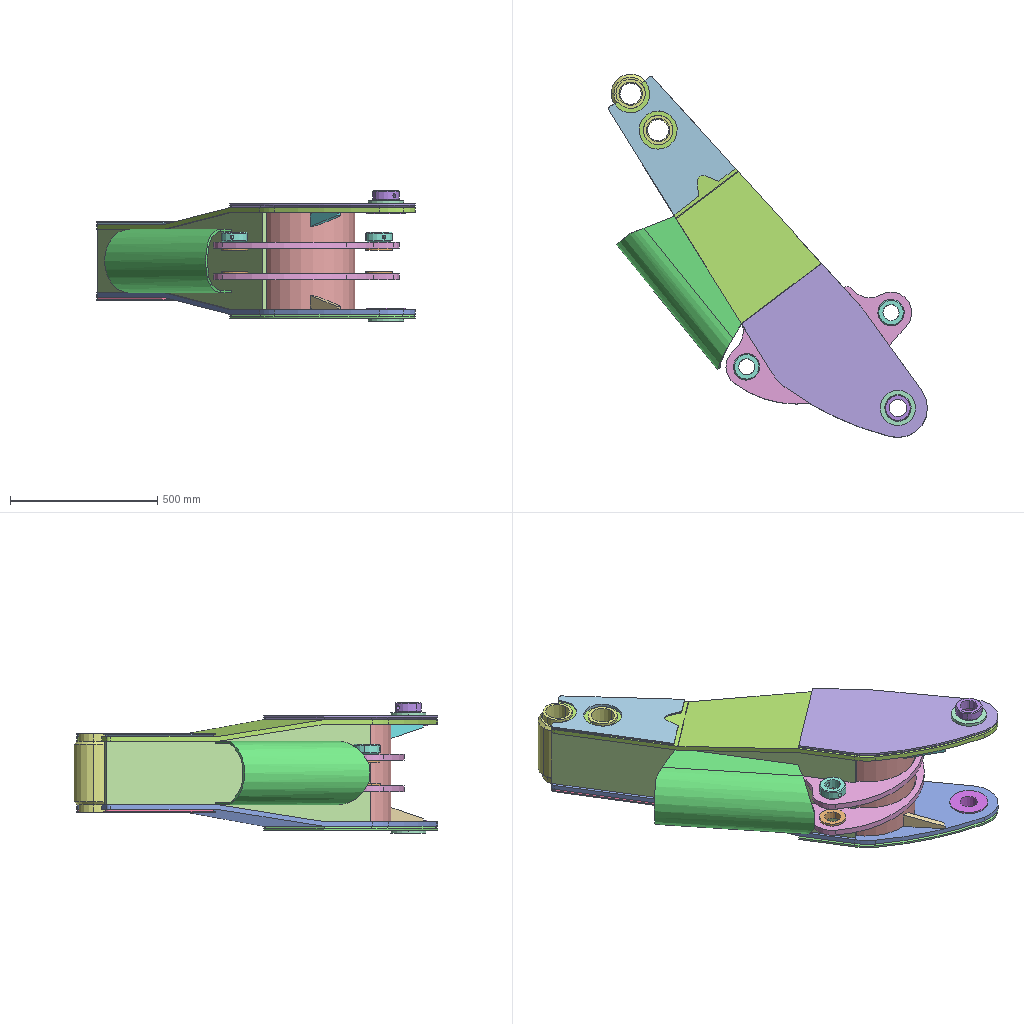Assembly | SolidWorks | 21 different items | 30 placed | box 1082 x 1232 x 444 mm
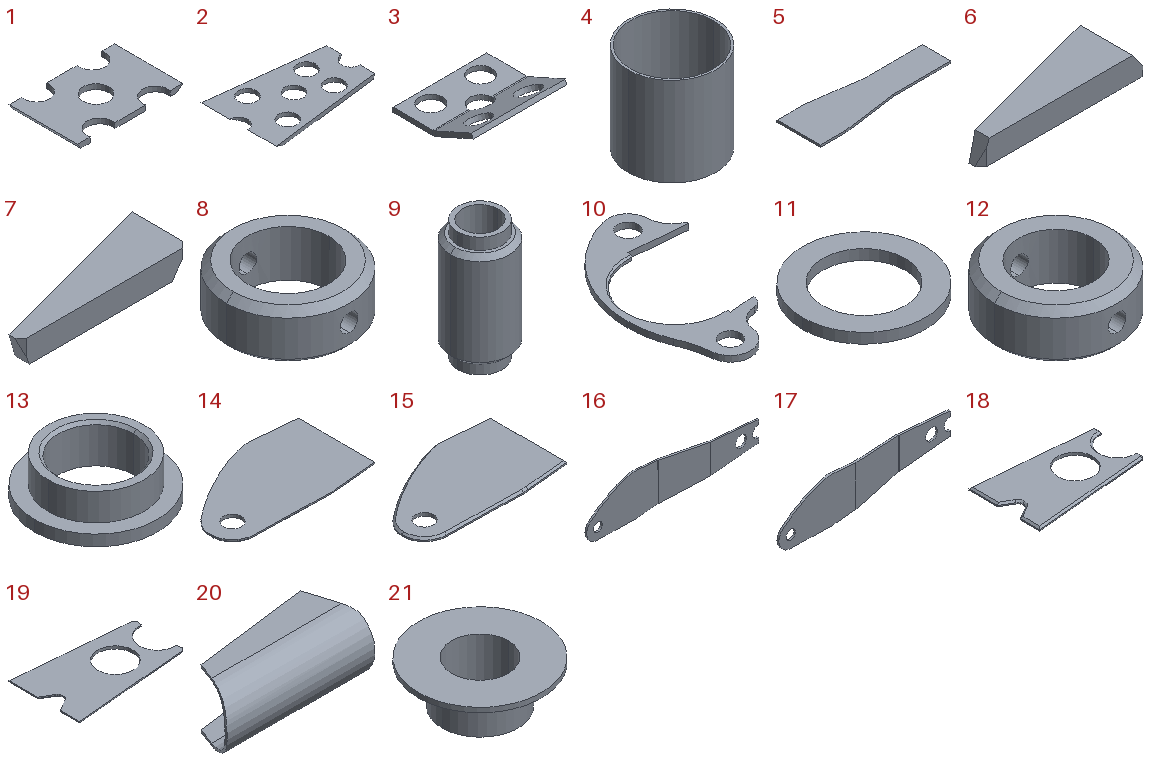Parts list (item | quantity | size | volume | features):
1 | x1 | 333 x 216 x 16 mm | 816357 mm3 | features Extrusion 1, ICE 1
2 | x1 | 489.6 x 328 x 16 mm | 1548186 mm3 | features Extrusion 1, ICE 1
3 | x1 | 330 x 281.818 x 74.519 mm | 1134363 mm3 | features FlatPattern 1, SM3dBend 1, SMBaseFlange 1, SheetMetal 1
4 | x1 | 325 x 325 x 330 mm | 2629136 mm3 | features Extrusion 1
5 | x2 | 1056 x 330 x 16 mm | 4392263 mm3 | features Extrusion 1
6 | x1 | 142.6 x 48 x 20 mm | 75242 mm3 | features Extrusion 1, ICE 1
7 | x1 | 142.6 x 48 x 20 mm | 75242 mm3 | features Extrusion 1, ICE 1
8 | x1 | 90 x 90 x 34 mm | 111520 mm3 | features Chamfer 2, Extrusion 1, ICE 1
9 | x2 | 133 x 133 x 268 mm | 2114999 mm3 | features ICE 5, Chamfer 2, Extrusion 1
10 | x2 | 398.626 x 642.2 x 20 mm | 1286836 mm3 | features Chamfer 1, Extrusion 1
11 | x2 | 120 x 120 x 10 mm | 62832 mm3 | features Extrusion 1
12 | x2 | 90 x 90 x 34 mm | 126206 mm3 | features Chamfer 2, Extrusion 1, ICE 1
13 | x4 | 90 x 90 x 28 mm | 60986 mm3 | features Chamfer 1, Extrusion 1, ICE 1
14 | x1 | 647.5 x 377 x 14 mm | 2654377 mm3 | features Chamfer 1, Extrusion 1
15 | x1 | 647.5 x 377 x 14 mm | 2654377 mm3 | features Chamfer 1, Extrusion 1
16 | x1 | 1506 x 73 x 377 mm | 6517874 mm3 | features Extrusion 1, ICE 1
17 | x1 | 1506 x 73 x 377 mm | 6517891 mm3 | features Extrusion 1, ICE 1
18 | x1 | 424.836 x 261.6 x 10 mm | 684949 mm3 | features Chamfer 1, Extrusion 1
19 | x1 | 424.836 x 261.6 x 10 mm | 684949 mm3 | features Chamfer 1, Extrusion 1
20 | x1 | 545.7 x 223.987 x 216 mm | 2017501 mm3 | features FlatPattern 1, SM3dBend 1, SMBaseFlange 1, SheetMetal 1
21 | x2 | 130 x 130 x 45 mm | 140194 mm3 | features Extrusion 1, ICE 1
Mates (type | each side: item.copy, entity, surface, feature):
Concentric | 4.1 face cylinder Boss-Extrude1 | 16.1 face cylinder Cut-Extrude1
Coincident | 4.1 face plane Boss-Extrude1 | 16.1 face plane Boss-Extrude1
Concentric | 4.1 face cylinder Boss-Extrude1 | 17.1 face cylinder Cut-Extrude1
Coincident | 4.1 face plane Boss-Extrude1 | 17.1 face plane Boss-Extrude1
Concentric | 16.1 face cylinder Cut-Extrude1 | 17.1 face cylinder Cut-Extrude1
Concentric | 4.1 face cylinder Boss-Extrude1 | 10.1 face cylinder Boss-Extrude1
Concentric | 4.1 face cylinder Boss-Extrude1 | 10.2 face cylinder Boss-Extrude1
DistanceDim | 10.2 face plane Boss-Extrude1 | 10.1 face plane Boss-Extrude1
DistanceDim | 10.2 face plane Boss-Extrude1 | 16.1 face plane Boss-Extrude1
Concentric | 10.2 face cylinder Boss-Extrude1 | 10.1 face cylinder Boss-Extrude1
Concentric | 10.2 face cylinder Boss-Extrude1 | 13.1 face cylinder Cut-Extrude1
Coincident | 10.2 face plane Boss-Extrude1 | 13.1 face plane Cut-Extrude1
Concentric | 10.1 face cylinder Boss-Extrude1 | 13.2 face cylinder Cut-Extrude1
Coincident | 10.1 face plane Boss-Extrude1 | 13.2 face plane Cut-Extrude1
Concentric | 12.1 face cylinder Boss-Extrude1 | 13.2 face cylinder Boss-Extrude1
Coincident | 10.1 face plane Boss-Extrude1 | 12.1 face plane Boss-Extrude1
Concentric | 10.2 face cylinder Boss-Extrude1 | 13.3 face cylinder Boss-Extrude1
Coincident | 10.2 face plane Boss-Extrude1 | 13.3 face plane Cut-Extrude1
Concentric | 10.1 face cylinder Boss-Extrude1 | 13.4 face cylinder Cut-Extrude1
Coincident | 10.1 face plane Boss-Extrude1 | 13.4 face plane Cut-Extrude1
Concentric | 12.2 face cylinder Boss-Extrude1 | 13.4 face cylinder Boss-Extrude1
Coincident | 10.1 face plane Boss-Extrude1 | 12.2 face plane Boss-Extrude1
Parallel | 17.1 face plane Cut-Extrude1 | 10.1 face plane Boss-Extrude1
Concentric | 16.1 face cylinder Cut-Extrude1 | 15.1 face cylinder Boss-Extrude1
Coincident | 16.1 face plane Boss-Extrude1 | 15.1 face plane Boss-Extrude1
Parallel | 16.1 face plane Cut-Extrude1 | 15.1 face plane Boss-Extrude1
Concentric | 17.1 face cylinder Cut-Extrude1 | 14.1 face cylinder Boss-Extrude1
Coincident | 17.1 face plane Boss-Extrude1 | 14.1 face plane Boss-Extrude1
Parallel | 17.1 face plane Cut-Extrude1 | 14.1 face plane Boss-Extrude1
Coincident | 16.1 face plane Boss-Extrude1 | 18.1 face plane Boss-Extrude1
Concentric | 16.1 face cylinder Cut-Extrude1 | 18.1 face cylinder Boss-Extrude1 | 2 times
Coincident | 17.1 face plane Boss-Extrude1 | 19.1 face plane Boss-Extrude1
Concentric | 17.1 face cylinder Cut-Extrude1 | 19.1 face cylinder Boss-Extrude1 | 2 times
Concentric | 17.1 face cylinder Cut-Extrude1 | 9.1 face cylinder Cut-Extrude1
Coincident | 19.1 face plane Boss-Extrude1 | 9.1 face plane Boss-Extrude3
Concentric | 17.1 face cylinder Cut-Extrude1 | 9.2 face cylinder Boss-Extrude3
Coincident | 19.1 face plane Boss-Extrude1 | 9.2 face plane Boss-Extrude3
Concentric | 14.1 face cylinder Boss-Extrude1 | 21.1 face cylinder Boss-Extrude1
Coincident | 17.1 face plane Boss-Extrude1 | 21.1 face plane Boss-Extrude2
Concentric | 21.1 face cylinder Boss-Extrude1 | 11.1 face cylinder Boss-Extrude1
Coincident | 14.1 face plane Boss-Extrude1 | 11.1 face plane Boss-Extrude1
Coincident | 16.1 face plane Boss-Extrude1 | 21.2 face plane Boss-Extrude2
Concentric | 16.1 face cylinder Cut-Extrude1 | 21.2 face cylinder Boss-Extrude1
Concentric | 21.2 face cylinder Boss-Extrude1 | 11.2 face cylinder Boss-Extrude1
Coincident | 15.1 face plane Boss-Extrude1 | 11.2 face plane Boss-Extrude1
DistanceDim | 5.1 face plane Boss-Extrude1 | 17.1 face plane Cut-Extrude1
Coincident | 17.1 face plane Boss-Extrude1 | 5.1 face plane Boss-Extrude1
Coincident | 10.2 face plane Boss-Extrude1 | 5.1 edge
Coincident | 2.1 face plane Cut-Extrude2 | 5.1 face plane Boss-Extrude1
Coincident | 1.1 face plane Cut-Extrude1 | 5.1 face plane Boss-Extrude1
Coincident | 16.1 face plane Boss-Extrude1 | 1.1 face plane Boss-Extrude1
Tangent | 9.1 face cylinder Boss-Extrude2 | 1.1 face plane Boss-Extrude1
Parallel | 1.1 edge | 2.1 edge
Coincident | 1.1 face plane Cut-Extrude1 | 2.1 vertex
Coincident | 17.1 face plane Boss-Extrude1 | 2.1 vertex
Coincident | 17.1 face plane Boss-Extrude1 | 3.1 face plane Base-Flange1
Coincident | 17.1 edge | 3.1 vertex | 2 times
Coincident | 5.1 face plane Boss-Extrude1 | 3.1 edge
Coincident | 16.1 face plane Boss-Extrude1 | 6.1 face plane Boss-Extrude1
Tangent | 4.1 face cylinder Boss-Extrude1 | 6.1 face plane Cut-Extrude1
Coincident | 16.1 face cylinder Cut-Extrude1 | 6.1 edge
Coincident | 4.1 face cylinder Boss-Extrude1 | 6.1 vertex
Coincident | 17.1 face plane Boss-Extrude1 | 7.1 face plane Boss-Extrude1
Tangent | 4.1 face cylinder Boss-Extrude1 | 7.1 face plane Cut-Extrude2
Coincident | 17.1 face cylinder Cut-Extrude1 | 7.1 edge
Coincident | 4.1 face cylinder Boss-Extrude1 | 7.1 vertex
Coincident | 16.1 face plane Boss-Extrude1 | 5.2 face plane Boss-Extrude1
Coincident | 10.1 face plane Boss-Extrude1 | 5.2 face plane Boss-Extrude1
Coincident | 10.2 face plane Boss-Extrude1 | 5.2 edge
Concentric | 21.1 face cylinder Boss-Extrude1 | 8.1 face cylinder Boss-Extrude1
Coincident | 8.1 face plane Boss-Extrude1 | 11.1 face plane Boss-Extrude1
Coincident | 17.1 face plane Boss-Extrude1 | 20.1 face plane Base-Flange1
Coincident | 5.2 face plane Boss-Extrude1 | 20.1 face plane Base-Flange1
DistanceDim | 20.1 edge | 5.2 edge